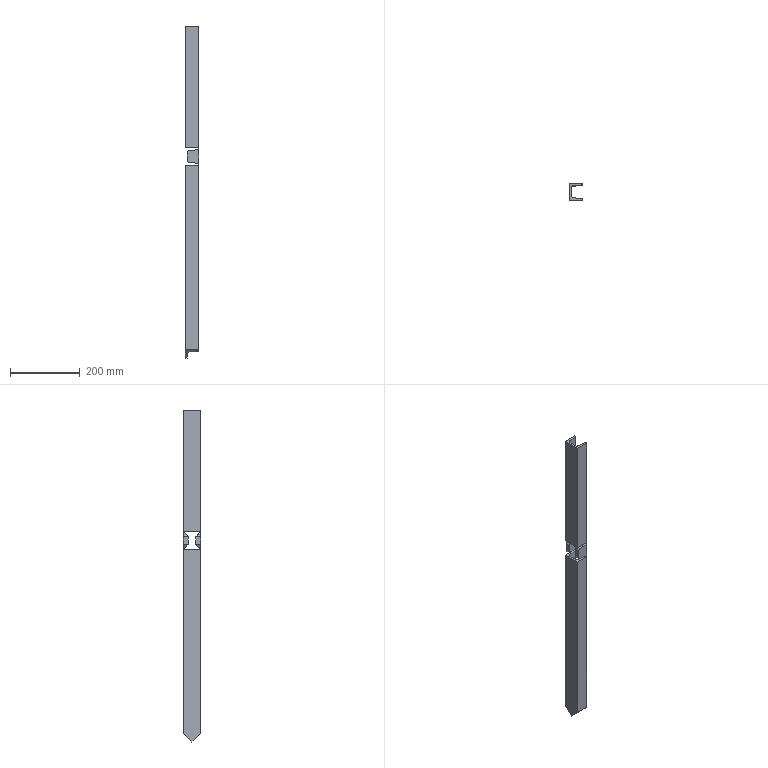Part | STEP file | DIN 1026-1 U 50 1785357074616 | 4 solids | 53 faces | box 38 x 50 x 953.851 mm | volume 646774 mm3 | plane 33 | cylinder 20 | commonest cylinder face diameters 7 x10 14 x10
STEP:
#1=CARTESIAN_POINT('',(38.,25.,556.1));
#2=VERTEX_POINT('',#1);
#3=CARTESIAN_POINT('',(34.779,25.,559.589));
#4=VERTEX_POINT('',#3);
#5=CARTESIAN_POINT('',(34.5,25.,556.1));
#6=DIRECTION('',(0.,-1.,0.));
#7=DIRECTION('',(-0.07975,0.,-0.9968));
#8=AXIS2_PLACEMENT_3D('',#5,#6,#7);
#9=CIRCLE('',#8,3.5);
#10=EDGE_CURVE('',#2,#4,#9,.T.);
#11=ORIENTED_EDGE('',*,*,#10,.F.);
#12=CARTESIAN_POINT('',(38.,22.751,556.1));
#13=VERTEX_POINT('',#12);
#14=CARTESIAN_POINT('',(38.,-253.555,556.1));
#15=DIRECTION('',(0.,1.,0.));
#16=VECTOR('',#15,10.);
#17=LINE('',#14,#16);
#18=EDGE_CURVE('',#13,#2,#17,.T.);
#19=ORIENTED_EDGE('',*,*,#18,.F.);
#20=CARTESIAN_POINT('',(34.779,19.262,559.589));
#21=VERTEX_POINT('',#20);
#22=CARTESIAN_POINT('',(34.5,22.751,556.1));
#23=DIRECTION('',(0.,0.7071,0.7071));
#24=DIRECTION('',(0.,0.7071,-0.7071));
#25=AXIS2_PLACEMENT_3D('',#22,#23,#24);
#26=ELLIPSE('',#25,4.95,3.5);
#27=EDGE_CURVE('',#21,#13,#26,.T.);
#28=ORIENTED_EDGE('',*,*,#27,.F.);
#29=CARTESIAN_POINT('',(34.779,-253.555,559.589));
#30=DIRECTION('',(0.,-1.,0.));
#31=VECTOR('',#30,10.);
#32=LINE('',#29,#31);
#33=EDGE_CURVE('',#4,#21,#32,.T.);
#34=ORIENTED_EDGE('',*,*,#33,.F.);
#35=EDGE_LOOP('',(#11,#19,#28,#34));
#36=FACE_OUTER_BOUND('',#35,.T.);
#37=CARTESIAN_POINT('',(34.5,-253.555,556.1));
#38=DIRECTION('',(0.,1.,0.));
#39=DIRECTION('',(-0.07975,0.,-0.9968));
#40=AXIS2_PLACEMENT_3D('',#37,#38,#39);
#41=CYLINDRICAL_SURFACE('',#40,3.5);
#42=ADVANCED_FACE('',(#36),#41,.F.);
#43=CARTESIAN_POINT('',(11.442,25.,561.456));
#44=VERTEX_POINT('',#43);
#45=CARTESIAN_POINT('',(28.073,25.,560.126));
#46=DIRECTION('',(-0.9968,0.,0.07975));
#47=VECTOR('',#46,10.);
#48=LINE('',#45,#47);
#49=EDGE_CURVE('',#4,#44,#48,.T.);
#50=ORIENTED_EDGE('',*,*,#49,.F.);
#51=ORIENTED_EDGE('',*,*,#33,.T.);
#52=CARTESIAN_POINT('',(11.442,17.395,561.456));
#53=VERTEX_POINT('',#52);
#54=CARTESIAN_POINT('',(34.51,19.241,559.611));
#55=DIRECTION('',(0.9937,0.07949,-0.07949));
#56=VECTOR('',#55,10.);
#57=LINE('',#54,#56);
#58=EDGE_CURVE('',#53,#21,#57,.T.);
#59=ORIENTED_EDGE('',*,*,#58,.F.);
#60=CARTESIAN_POINT('',(11.442,-253.555,561.456));
#61=DIRECTION('',(0.,-1.,0.));
#62=VECTOR('',#61,10.);
#63=LINE('',#60,#62);
#64=EDGE_CURVE('',#44,#53,#63,.T.);
#65=ORIENTED_EDGE('',*,*,#64,.F.);
#66=EDGE_LOOP('',(#50,#51,#59,#65));
#67=FACE_OUTER_BOUND('',#66,.T.);
#68=CARTESIAN_POINT('',(11.442,-253.555,561.456));
#69=DIRECTION('',(0.07975,0.,0.9968));
#70=DIRECTION('',(0.9968,0.,-0.07975));
#71=AXIS2_PLACEMENT_3D('',#68,#69,#70);
#72=PLANE('',#71);
#73=ADVANCED_FACE('',(#67),#72,.F.);
#74=CARTESIAN_POINT('',(5.,25.,568.434));
#75=VERTEX_POINT('',#74);
#76=CARTESIAN_POINT('',(12.,25.,568.434));
#77=DIRECTION('',(0.,1.,0.));
#78=DIRECTION('',(-0.07975,0.,-0.9968));
#79=AXIS2_PLACEMENT_3D('',#76,#77,#78);
#80=CIRCLE('',#79,7.);
#81=EDGE_CURVE('',#44,#75,#80,.T.);
#82=ORIENTED_EDGE('',*,*,#81,.F.);
#83=ORIENTED_EDGE('',*,*,#64,.T.);
#84=CARTESIAN_POINT('',(5.,10.418,568.434));
#85=VERTEX_POINT('',#84);
#86=CARTESIAN_POINT('',(12.,10.418,568.434));
#87=DIRECTION('',(0.,-0.7071,-0.7071));
#88=DIRECTION('',(0.,0.7071,-0.7071));
#89=AXIS2_PLACEMENT_3D('',#86,#87,#88);
#90=ELLIPSE('',#89,9.899,7.);
#91=EDGE_CURVE('',#85,#53,#90,.T.);
#92=ORIENTED_EDGE('',*,*,#91,.F.);
#93=CARTESIAN_POINT('',(5.,-253.555,568.434));
#94=DIRECTION('',(0.,-1.,0.));
#95=VECTOR('',#94,10.);
#96=LINE('',#93,#95);
#97=EDGE_CURVE('',#75,#85,#96,.T.);
#98=ORIENTED_EDGE('',*,*,#97,.F.);
#99=EDGE_LOOP('',(#82,#83,#92,#98));
#100=FACE_OUTER_BOUND('',#99,.T.);
#101=CARTESIAN_POINT('',(12.,-253.555,568.434));
#102=DIRECTION('',(0.,1.,0.));
#103=DIRECTION('',(-0.07975,0.,-0.9968));
#104=AXIS2_PLACEMENT_3D('',#101,#102,#103);
#105=CYLINDRICAL_SURFACE('',#104,7.);
#106=ADVANCED_FACE('',(#100),#105,.T.);
#107=CARTESIAN_POINT('',(5.,25.,589.269));
#108=VERTEX_POINT('',#107);
#109=CARTESIAN_POINT('',(5.,25.,294.634));
#110=DIRECTION('',(0.,0.,1.));
#111=VECTOR('',#110,10.);
#112=LINE('',#109,#111);
#113=EDGE_CURVE('',#75,#108,#112,.T.);
#114=ORIENTED_EDGE('',*,*,#113,.F.);
#115=ORIENTED_EDGE('',*,*,#97,.T.);
#116=CARTESIAN_POINT('',(5.,10.418,589.269));
#117=VERTEX_POINT('',#116);
#118=CARTESIAN_POINT('',(5.,10.418,0.));
#119=DIRECTION('',(0.,0.,1.));
#120=VECTOR('',#119,10.);
#121=LINE('',#118,#120);
#122=EDGE_CURVE('',#85,#117,#121,.T.);
#123=ORIENTED_EDGE('',*,*,#122,.T.);
#124=CARTESIAN_POINT('',(5.,-253.555,589.269));
#125=DIRECTION('',(0.,-1.,0.));
#126=VECTOR('',#125,10.);
#127=LINE('',#124,#126);
#128=EDGE_CURVE('',#108,#117,#127,.T.);
#129=ORIENTED_EDGE('',*,*,#128,.F.);
#130=EDGE_LOOP('',(#114,#115,#123,#129));
#131=FACE_OUTER_BOUND('',#130,.T.);
#132=CARTESIAN_POINT('',(5.,-253.555,589.269));
#133=DIRECTION('',(1.,0.,0.));
#134=DIRECTION('',(0.,0.,-1.));
#135=AXIS2_PLACEMENT_3D('',#132,#133,#134);
#136=PLANE('',#135);
#137=ADVANCED_FACE('',(#131),#136,.F.);
#138=CARTESIAN_POINT('',(11.442,25.,596.247));
#139=VERTEX_POINT('',#138);
#140=CARTESIAN_POINT('',(12.,25.,589.269));
#141=DIRECTION('',(0.,1.,0.));
#142=DIRECTION('',(-1.,0.,0.));
#143=AXIS2_PLACEMENT_3D('',#140,#141,#142);
#144=CIRCLE('',#143,7.);
#145=EDGE_CURVE('',#108,#139,#144,.T.);
#146=ORIENTED_EDGE('',*,*,#145,.F.);
#147=ORIENTED_EDGE('',*,*,#128,.T.);
#148=CARTESIAN_POINT('',(11.442,17.395,596.247));
#149=VERTEX_POINT('',#148);
#150=CARTESIAN_POINT('',(12.,10.418,589.269));
#151=DIRECTION('',(0.,-0.7071,0.7071));
#152=DIRECTION('',(0.,0.7071,0.7071));
#153=AXIS2_PLACEMENT_3D('',#150,#151,#152);
#154=ELLIPSE('',#153,9.899,7.);
#155=EDGE_CURVE('',#149,#117,#154,.T.);
#156=ORIENTED_EDGE('',*,*,#155,.F.);
#157=CARTESIAN_POINT('',(11.442,-253.555,596.247));
#158=DIRECTION('',(0.,-1.,0.));
#159=VECTOR('',#158,10.);
#160=LINE('',#157,#159);
#161=EDGE_CURVE('',#139,#149,#160,.T.);
#162=ORIENTED_EDGE('',*,*,#161,.F.);
#163=EDGE_LOOP('',(#146,#147,#156,#162));
#164=FACE_OUTER_BOUND('',#163,.T.);
#165=CARTESIAN_POINT('',(12.,-253.555,589.269));
#166=DIRECTION('',(0.,1.,0.));
#167=DIRECTION('',(-1.,0.,0.));
#168=AXIS2_PLACEMENT_3D('',#165,#166,#167);
#169=CYLINDRICAL_SURFACE('',#168,7.);
#170=ADVANCED_FACE('',(#164),#169,.T.);
#171=CARTESIAN_POINT('',(34.779,25.,598.114));
#172=VERTEX_POINT('',#171);
#173=CARTESIAN_POINT('',(38.,25.,601.603));
#174=VERTEX_POINT('',#173);
#175=CARTESIAN_POINT('',(34.5,25.,601.603));
#176=DIRECTION('',(0.,-1.,0.));
#177=DIRECTION('',(-1.,0.,0.));
#178=AXIS2_PLACEMENT_3D('',#175,#176,#177);
#179=CIRCLE('',#178,3.5);
#180=EDGE_CURVE('',#172,#174,#179,.T.);
#181=ORIENTED_EDGE('',*,*,#180,.F.);
#182=CARTESIAN_POINT('',(34.779,19.262,598.114));
#183=VERTEX_POINT('',#182);
#184=CARTESIAN_POINT('',(34.779,-253.555,598.114));
#185=DIRECTION('',(0.,-1.,0.));
#186=VECTOR('',#185,10.);
#187=LINE('',#184,#186);
#188=EDGE_CURVE('',#172,#183,#187,.T.);
#189=ORIENTED_EDGE('',*,*,#188,.T.);
#190=CARTESIAN_POINT('',(38.,22.751,601.603));
#191=VERTEX_POINT('',#190);
#192=CARTESIAN_POINT('',(34.5,22.751,601.603));
#193=DIRECTION('',(0.,0.7071,-0.7071));
#194=DIRECTION('',(0.,0.7071,0.7071));
#195=AXIS2_PLACEMENT_3D('',#192,#193,#194);
#196=ELLIPSE('',#195,4.95,3.5);
#197=EDGE_CURVE('',#191,#183,#196,.T.);
#198=ORIENTED_EDGE('',*,*,#197,.F.);
#199=CARTESIAN_POINT('',(38.,-253.555,601.603));
#200=DIRECTION('',(0.,1.,0.));
#201=VECTOR('',#200,10.);
#202=LINE('',#199,#201);
#203=EDGE_CURVE('',#191,#174,#202,.T.);
#204=ORIENTED_EDGE('',*,*,#203,.T.);
#205=EDGE_LOOP('',(#181,#189,#198,#204));
#206=FACE_OUTER_BOUND('',#205,.T.);
#207=CARTESIAN_POINT('',(34.5,-253.555,601.603));
#208=DIRECTION('',(0.,1.,0.));
#209=DIRECTION('',(-1.,0.,0.));
#210=AXIS2_PLACEMENT_3D('',#207,#208,#209);
#211=CYLINDRICAL_SURFACE('',#210,3.5);
#212=ADVANCED_FACE('',(#206),#211,.F.);
#213=CARTESIAN_POINT('',(-6.272,25.,594.83));
#214=DIRECTION('',(0.9968,0.,0.07975));
#215=VECTOR('',#214,10.);
#216=LINE('',#213,#215);
#217=EDGE_CURVE('',#139,#172,#216,.T.);
#218=ORIENTED_EDGE('',*,*,#217,.F.);
#219=ORIENTED_EDGE('',*,*,#161,.T.);
#220=CARTESIAN_POINT('',(0.3821,16.511,595.362));
#221=DIRECTION('',(-0.9937,-0.07949,-0.07949));
#222=VECTOR('',#221,10.);
#223=LINE('',#220,#222);
#224=EDGE_CURVE('',#183,#149,#223,.T.);
#225=ORIENTED_EDGE('',*,*,#224,.F.);
#226=ORIENTED_EDGE('',*,*,#188,.F.);
#227=EDGE_LOOP('',(#218,#219,#225,#226));
#228=FACE_OUTER_BOUND('',#227,.T.);
#229=CARTESIAN_POINT('',(34.779,-253.555,598.114));
#230=DIRECTION('',(0.07975,0.,-0.9968));
#231=DIRECTION('',(-0.9968,0.,-0.07975));
#232=AXIS2_PLACEMENT_3D('',#229,#230,#231);
#233=PLANE('',#232);
#234=ADVANCED_FACE('',(#228),#233,.F.);
#235=ORIENTED_EDGE('',*,*,#10,.T.);
#236=ORIENTED_EDGE('',*,*,#49,.T.);
#237=ORIENTED_EDGE('',*,*,#81,.T.);
#238=ORIENTED_EDGE('',*,*,#113,.T.);
#239=ORIENTED_EDGE('',*,*,#145,.T.);
#240=ORIENTED_EDGE('',*,*,#217,.T.);
#241=ORIENTED_EDGE('',*,*,#180,.T.);
#242=CARTESIAN_POINT('',(38.,25.,0.));
#243=DIRECTION('',(0.,0.,1.));
#244=VECTOR('',#243,10.);
#245=LINE('',#242,#244);
#246=EDGE_CURVE('',#2,#174,#245,.T.);
#247=ORIENTED_EDGE('',*,*,#246,.F.);
#248=EDGE_LOOP('',(#235,#236,#237,#238,#239,#240,#241,#247));
#249=FACE_OUTER_BOUND('',#248,.T.);
#250=CARTESIAN_POINT('',(0.,25.,0.));
#251=DIRECTION('',(0.,1.,0.));
#252=DIRECTION('',(0.,0.,1.));
#253=AXIS2_PLACEMENT_3D('',#250,#251,#252);
#254=PLANE('',#253);
#255=ADVANCED_FACE('',(#249),#254,.T.);
#256=ORIENTED_EDGE('',*,*,#18,.T.);
#257=ORIENTED_EDGE('',*,*,#246,.T.);
#258=ORIENTED_EDGE('',*,*,#203,.F.);
#259=CARTESIAN_POINT('',(38.,22.751,0.));
#260=DIRECTION('',(0.,0.,1.));
#261=VECTOR('',#260,10.);
#262=LINE('',#259,#261);
#263=EDGE_CURVE('',#13,#191,#262,.T.);
#264=ORIENTED_EDGE('',*,*,#263,.F.);
#265=EDGE_LOOP('',(#256,#257,#258,#264));
#266=FACE_OUTER_BOUND('',#265,.T.);
#267=CARTESIAN_POINT('',(38.,25.,0.));
#268=DIRECTION('',(1.,0.,0.));
#269=DIRECTION('',(0.,0.,-1.));
#270=AXIS2_PLACEMENT_3D('',#267,#268,#269);
#271=PLANE('',#270);
#272=ADVANCED_FACE('',(#266),#271,.T.);
#273=ORIENTED_EDGE('',*,*,#91,.T.);
#274=CARTESIAN_POINT('',(11.442,17.395,0.));
#275=DIRECTION('',(0.,0.,1.));
#276=VECTOR('',#275,10.);
#277=LINE('',#274,#276);
#278=EDGE_CURVE('',#53,#149,#277,.T.);
#279=ORIENTED_EDGE('',*,*,#278,.T.);
#280=ORIENTED_EDGE('',*,*,#155,.T.);
#281=ORIENTED_EDGE('',*,*,#122,.F.);
#282=EDGE_LOOP('',(#273,#279,#280,#281));
#283=FACE_OUTER_BOUND('',#282,.T.);
#284=CARTESIAN_POINT('',(12.,10.418,0.));
#285=DIRECTION('',(0.,0.,1.));
#286=DIRECTION('',(-0.07975,0.9968,0.));
#287=AXIS2_PLACEMENT_3D('',#284,#285,#286);
#288=CYLINDRICAL_SURFACE('',#287,7.);
#289=ADVANCED_FACE('',(#283),#288,.F.);
#290=ORIENTED_EDGE('',*,*,#27,.T.);
#291=ORIENTED_EDGE('',*,*,#263,.T.);
#292=ORIENTED_EDGE('',*,*,#197,.T.);
#293=CARTESIAN_POINT('',(34.779,19.262,0.));
#294=DIRECTION('',(0.,0.,1.));
#295=VECTOR('',#294,10.);
#296=LINE('',#293,#295);
#297=EDGE_CURVE('',#21,#183,#296,.T.);
#298=ORIENTED_EDGE('',*,*,#297,.F.);
#299=EDGE_LOOP('',(#290,#291,#292,#298));
#300=FACE_OUTER_BOUND('',#299,.T.);
#301=CARTESIAN_POINT('',(34.5,22.751,0.));
#302=DIRECTION('',(0.,0.,1.));
#303=DIRECTION('',(-0.07975,0.9968,0.));
#304=AXIS2_PLACEMENT_3D('',#301,#302,#303);
#305=CYLINDRICAL_SURFACE('',#304,3.5);
#306=ADVANCED_FACE('',(#300),#305,.T.);
#307=ORIENTED_EDGE('',*,*,#58,.T.);
#308=ORIENTED_EDGE('',*,*,#297,.T.);
#309=ORIENTED_EDGE('',*,*,#224,.T.);
#310=ORIENTED_EDGE('',*,*,#278,.F.);
#311=EDGE_LOOP('',(#307,#308,#309,#310));
#312=FACE_OUTER_BOUND('',#311,.T.);
#313=CARTESIAN_POINT('',(34.779,19.262,0.));
#314=DIRECTION('',(0.07975,-0.9968,0.));
#315=DIRECTION('',(0.,0.,-1.));
#316=AXIS2_PLACEMENT_3D('',#313,#314,#315);
#317=PLANE('',#316);
#318=ADVANCED_FACE('',(#312),#317,.T.);
#319=CLOSED_SHELL('',(#42,#73,#106,#137,#170,#212,#234,#255,#272,#289,#306,#318));
#320=MANIFOLD_SOLID_BREP('',#319);
#321=CARTESIAN_POINT('',(5.,0.,0.));
#322=VERTEX_POINT('',#321);
#323=CARTESIAN_POINT('',(0.,0.,0.));
#324=VERTEX_POINT('',#323);
#325=CARTESIAN_POINT('',(9.5,0.,0.));
#326=DIRECTION('',(-1.,0.,0.));
#327=VECTOR('',#326,10.);
#328=LINE('',#325,#327);
#329=EDGE_CURVE('',#322,#324,#328,.T.);
#330=ORIENTED_EDGE('',*,*,#329,.T.);
#331=CARTESIAN_POINT('',(0.,25.,25.));
#332=VERTEX_POINT('',#331);
#333=CARTESIAN_POINT('',(0.,0.,0.));
#334=DIRECTION('',(0.,-0.7071,-0.7071));
#335=VECTOR('',#334,10.);
#336=LINE('',#333,#335);
#337=EDGE_CURVE('',#332,#324,#336,.T.);
#338=ORIENTED_EDGE('',*,*,#337,.F.);
#339=CARTESIAN_POINT('',(38.,25.,25.));
#340=VERTEX_POINT('',#339);
#341=CARTESIAN_POINT('',(0.,25.,25.));
#342=DIRECTION('',(-1.,0.,0.));
#343=VECTOR('',#342,10.);
#344=LINE('',#341,#343);
#345=EDGE_CURVE('',#340,#332,#344,.T.);
#346=ORIENTED_EDGE('',*,*,#345,.F.);
#347=CARTESIAN_POINT('',(38.,22.751,22.751));
#348=VERTEX_POINT('',#347);
#349=CARTESIAN_POINT('',(38.,6.25,6.25));
#350=DIRECTION('',(0.,0.7071,0.7071));
#351=VECTOR('',#350,10.);
#352=LINE('',#349,#351);
#353=EDGE_CURVE('',#348,#340,#352,.T.);
#354=ORIENTED_EDGE('',*,*,#353,.F.);
#355=CARTESIAN_POINT('',(34.779,19.262,19.262));
#356=VERTEX_POINT('',#355);
#357=CARTESIAN_POINT('',(34.5,22.751,22.751));
#358=DIRECTION('',(0.,-0.7071,0.7071));
#359=DIRECTION('',(0.,0.7071,0.7071));
#360=AXIS2_PLACEMENT_3D('',#357,#358,#359);
#361=ELLIPSE('',#360,4.95,3.5);
#362=EDGE_CURVE('',#356,#348,#361,.T.);
#363=ORIENTED_EDGE('',*,*,#362,.F.);
#364=CARTESIAN_POINT('',(11.442,17.395,17.395));
#365=VERTEX_POINT('',#364);
#366=CARTESIAN_POINT('',(15.327,17.706,17.706));
#367=DIRECTION('',(0.9937,0.07949,0.07949));
#368=VECTOR('',#367,10.);
#369=LINE('',#366,#368);
#370=EDGE_CURVE('',#365,#356,#369,.T.);
#371=ORIENTED_EDGE('',*,*,#370,.F.);
#372=CARTESIAN_POINT('',(5.,10.418,10.418));
#373=VERTEX_POINT('',#372);
#374=CARTESIAN_POINT('',(12.,10.418,10.418));
#375=DIRECTION('',(0.,0.7071,-0.7071));
#376=DIRECTION('',(0.,0.7071,0.7071));
#377=AXIS2_PLACEMENT_3D('',#374,#375,#376);
#378=ELLIPSE('',#377,9.899,7.);
#379=EDGE_CURVE('',#373,#365,#378,.T.);
#380=ORIENTED_EDGE('',*,*,#379,.F.);
#381=CARTESIAN_POINT('',(5.,0.,0.));
#382=DIRECTION('',(0.,0.7071,0.7071));
#383=VECTOR('',#382,10.);
#384=LINE('',#381,#383);
#385=EDGE_CURVE('',#322,#373,#384,.T.);
#386=ORIENTED_EDGE('',*,*,#385,.F.);
#387=EDGE_LOOP('',(#330,#338,#346,#354,#363,#371,#380,#386));
#388=FACE_OUTER_BOUND('',#387,.T.);
#389=CARTESIAN_POINT('',(0.,0.,0.));
#390=DIRECTION('',(0.,-0.7071,0.7071));
#391=DIRECTION('',(1.,0.,0.));
#392=AXIS2_PLACEMENT_3D('',#389,#390,#391);
#393=PLANE('',#392);
#394=ADVANCED_FACE('',(#388),#393,.F.);
#395=ORIENTED_EDGE('',*,*,#353,.T.);
#396=CARTESIAN_POINT('',(38.,25.,553.851));
#397=VERTEX_POINT('',#396);
#398=CARTESIAN_POINT('',(38.,25.,0.));
#399=DIRECTION('',(0.,0.,1.));
#400=VECTOR('',#399,10.);
#401=LINE('',#398,#400);
#402=EDGE_CURVE('',#340,#397,#401,.T.);
#403=ORIENTED_EDGE('',*,*,#402,.T.);
#404=CARTESIAN_POINT('',(38.,22.751,553.851));
#405=VERTEX_POINT('',#404);
#406=CARTESIAN_POINT('',(38.,-114.278,553.851));
#407=DIRECTION('',(0.,-1.,0.));
#408=VECTOR('',#407,10.);
#409=LINE('',#406,#408);
#410=EDGE_CURVE('',#397,#405,#409,.T.);
#411=ORIENTED_EDGE('',*,*,#410,.T.);
#412=CARTESIAN_POINT('',(38.,22.751,0.));
#413=DIRECTION('',(0.,0.,1.));
#414=VECTOR('',#413,10.);
#415=LINE('',#412,#414);
#416=EDGE_CURVE('',#348,#405,#415,.T.);
#417=ORIENTED_EDGE('',*,*,#416,.F.);
#418=EDGE_LOOP('',(#395,#403,#411,#417));
#419=FACE_OUTER_BOUND('',#418,.T.);
#420=CARTESIAN_POINT('',(38.,25.,0.));
#421=DIRECTION('',(1.,0.,0.));
#422=DIRECTION('',(0.,0.,-1.));
#423=AXIS2_PLACEMENT_3D('',#420,#421,#422);
#424=PLANE('',#423);
#425=ADVANCED_FACE('',(#419),#424,.T.);
#426=ORIENTED_EDGE('',*,*,#345,.T.);
#427=CARTESIAN_POINT('',(0.,25.,553.851));
#428=VERTEX_POINT('',#427);
#429=CARTESIAN_POINT('',(0.,25.,0.));
#430=DIRECTION('',(0.,0.,1.));
#431=VECTOR('',#430,10.);
#432=LINE('',#429,#431);
#433=EDGE_CURVE('',#332,#428,#432,.T.);
#434=ORIENTED_EDGE('',*,*,#433,.T.);
#435=CARTESIAN_POINT('',(19.,25.,553.851));
#436=DIRECTION('',(1.,0.,0.));
#437=VECTOR('',#436,10.);
#438=LINE('',#435,#437);
#439=EDGE_CURVE('',#428,#397,#438,.T.);
#440=ORIENTED_EDGE('',*,*,#439,.T.);
#441=ORIENTED_EDGE('',*,*,#402,.F.);
#442=EDGE_LOOP('',(#426,#434,#440,#441));
#443=FACE_OUTER_BOUND('',#442,.T.);
#444=CARTESIAN_POINT('',(0.,25.,0.));
#445=DIRECTION('',(0.,1.,0.));
#446=DIRECTION('',(0.,0.,1.));
#447=AXIS2_PLACEMENT_3D('',#444,#445,#446);
#448=PLANE('',#447);
#449=ADVANCED_FACE('',(#443),#448,.T.);
#450=ORIENTED_EDGE('',*,*,#337,.T.);
#451=CARTESIAN_POINT('',(0.,-25.,25.));
#452=VERTEX_POINT('',#451);
#453=CARTESIAN_POINT('',(0.,0.,0.));
#454=DIRECTION('',(0.,-0.7071,0.7071));
#455=VECTOR('',#454,10.);
#456=LINE('',#453,#455);
#457=EDGE_CURVE('',#324,#452,#456,.T.);
#458=ORIENTED_EDGE('',*,*,#457,.T.);
#459=CARTESIAN_POINT('',(0.,-25.,553.851));
#460=VERTEX_POINT('',#459);
#461=CARTESIAN_POINT('',(0.,-25.,0.));
#462=DIRECTION('',(0.,0.,1.));
#463=VECTOR('',#462,10.);
#464=LINE('',#461,#463);
#465=EDGE_CURVE('',#452,#460,#464,.T.);
#466=ORIENTED_EDGE('',*,*,#465,.T.);
#467=CARTESIAN_POINT('',(0.,-126.778,553.851));
#468=DIRECTION('',(0.,1.,0.));
#469=VECTOR('',#468,10.);
#470=LINE('',#467,#469);
#471=EDGE_CURVE('',#460,#428,#470,.T.);
#472=ORIENTED_EDGE('',*,*,#471,.T.);
#473=ORIENTED_EDGE('',*,*,#433,.F.);
#474=EDGE_LOOP('',(#450,#458,#466,#472,#473));
#475=FACE_OUTER_BOUND('',#474,.T.);
#476=CARTESIAN_POINT('',(0.,0.,0.));
#477=DIRECTION('',(-1.,0.,0.));
#478=DIRECTION('',(0.,0.,1.));
#479=AXIS2_PLACEMENT_3D('',#476,#477,#478);
#480=PLANE('',#479);
#481=ADVANCED_FACE('',(#475),#480,.T.);
#482=ORIENTED_EDGE('',*,*,#385,.T.);
#483=CARTESIAN_POINT('',(5.,10.418,553.851));
#484=VERTEX_POINT('',#483);
#485=CARTESIAN_POINT('',(5.,10.418,0.));
#486=DIRECTION('',(0.,0.,1.));
#487=VECTOR('',#486,10.);
#488=LINE('',#485,#487);
#489=EDGE_CURVE('',#373,#484,#488,.T.);
#490=ORIENTED_EDGE('',*,*,#489,.T.);
#491=CARTESIAN_POINT('',(5.,-10.418,553.851));
#492=VERTEX_POINT('',#491);
#493=CARTESIAN_POINT('',(5.,-126.778,553.851));
#494=DIRECTION('',(0.,-1.,0.));
#495=VECTOR('',#494,10.);
#496=LINE('',#493,#495);
#497=EDGE_CURVE('',#484,#492,#496,.T.);
#498=ORIENTED_EDGE('',*,*,#497,.T.);
#499=CARTESIAN_POINT('',(5.,-10.418,10.418));
#500=VERTEX_POINT('',#499);
#501=CARTESIAN_POINT('',(5.,-10.418,0.));
#502=DIRECTION('',(0.,0.,1.));
#503=VECTOR('',#502,10.);
#504=LINE('',#501,#503);
#505=EDGE_CURVE('',#500,#492,#504,.T.);
#506=ORIENTED_EDGE('',*,*,#505,.F.);
#507=CARTESIAN_POINT('',(5.,0.,0.));
#508=DIRECTION('',(0.,0.7071,-0.7071));
#509=VECTOR('',#508,10.);
#510=LINE('',#507,#509);
#511=EDGE_CURVE('',#500,#322,#510,.T.);
#512=ORIENTED_EDGE('',*,*,#511,.T.);
#513=EDGE_LOOP('',(#482,#490,#498,#506,#512));
#514=FACE_OUTER_BOUND('',#513,.T.);
#515=CARTESIAN_POINT('',(5.,0.,0.));
#516=DIRECTION('',(1.,0.,0.));
#517=DIRECTION('',(0.,0.,-1.));
#518=AXIS2_PLACEMENT_3D('',#515,#516,#517);
#519=PLANE('',#518);
#520=ADVANCED_FACE('',(#514),#519,.T.);
#521=ORIENTED_EDGE('',*,*,#379,.T.);
#522=CARTESIAN_POINT('',(11.442,17.395,553.851));
#523=VERTEX_POINT('',#522);
#524=CARTESIAN_POINT('',(11.442,17.395,0.));
#525=DIRECTION('',(0.,0.,1.));
#526=VECTOR('',#525,10.);
#527=LINE('',#524,#526);
#528=EDGE_CURVE('',#365,#523,#527,.T.);
#529=ORIENTED_EDGE('',*,*,#528,.T.);
#530=CARTESIAN_POINT('',(12.,10.418,553.851));
#531=DIRECTION('',(0.,0.,1.));
#532=DIRECTION('',(-0.07975,0.9968,0.));
#533=AXIS2_PLACEMENT_3D('',#530,#531,#532);
#534=CIRCLE('',#533,7.);
#535=EDGE_CURVE('',#523,#484,#534,.T.);
#536=ORIENTED_EDGE('',*,*,#535,.T.);
#537=ORIENTED_EDGE('',*,*,#489,.F.);
#538=EDGE_LOOP('',(#521,#529,#536,#537));
#539=FACE_OUTER_BOUND('',#538,.T.);
#540=CARTESIAN_POINT('',(12.,10.418,0.));
#541=DIRECTION('',(0.,0.,1.));
#542=DIRECTION('',(-0.07975,0.9968,0.));
#543=AXIS2_PLACEMENT_3D('',#540,#541,#542);
#544=CYLINDRICAL_SURFACE('',#543,7.);
#545=ADVANCED_FACE('',(#539),#544,.F.);
#546=ORIENTED_EDGE('',*,*,#370,.T.);
#547=CARTESIAN_POINT('',(34.779,19.262,553.851));
#548=VERTEX_POINT('',#547);
#549=CARTESIAN_POINT('',(34.779,19.262,0.));
#550=DIRECTION('',(0.,0.,1.));
#551=VECTOR('',#550,10.);
#552=LINE('',#549,#551);
#553=EDGE_CURVE('',#356,#548,#552,.T.);
#554=ORIENTED_EDGE('',*,*,#553,.T.);
#555=CARTESIAN_POINT('',(25.536,18.523,553.851));
#556=DIRECTION('',(-0.9968,-0.07975,0.));
#557=VECTOR('',#556,10.);
#558=LINE('',#555,#557);
#559=EDGE_CURVE('',#548,#523,#558,.T.);
#560=ORIENTED_EDGE('',*,*,#559,.T.);
#561=ORIENTED_EDGE('',*,*,#528,.F.);
#562=EDGE_LOOP('',(#546,#554,#560,#561));
#563=FACE_OUTER_BOUND('',#562,.T.);
#564=CARTESIAN_POINT('',(34.779,19.262,0.));
#565=DIRECTION('',(0.07975,-0.9968,0.));
#566=DIRECTION('',(0.,0.,-1.));
#567=AXIS2_PLACEMENT_3D('',#564,#565,#566);
#568=PLANE('',#567);
#569=ADVANCED_FACE('',(#563),#568,.T.);
#570=ORIENTED_EDGE('',*,*,#362,.T.);
#571=ORIENTED_EDGE('',*,*,#416,.T.);
#572=CARTESIAN_POINT('',(34.5,22.751,553.851));
#573=DIRECTION('',(0.,0.,-1.));
#574=DIRECTION('',(-0.07975,0.9968,0.));
#575=AXIS2_PLACEMENT_3D('',#572,#573,#574);
#576=CIRCLE('',#575,3.5);
#577=EDGE_CURVE('',#405,#548,#576,.T.);
#578=ORIENTED_EDGE('',*,*,#577,.T.);
#579=ORIENTED_EDGE('',*,*,#553,.F.);
#580=EDGE_LOOP('',(#570,#571,#578,#579));
#581=FACE_OUTER_BOUND('',#580,.T.);
#582=CARTESIAN_POINT('',(34.5,22.751,0.));
#583=DIRECTION('',(0.,0.,1.));
#584=DIRECTION('',(-0.07975,0.9968,0.));
#585=AXIS2_PLACEMENT_3D('',#582,#583,#584);
#586=CYLINDRICAL_SURFACE('',#585,3.5);
#587=ADVANCED_FACE('',(#581),#586,.T.);
#588=CARTESIAN_POINT('',(11.442,-17.395,17.395));
#589=VERTEX_POINT('',#588);
#590=CARTESIAN_POINT('',(12.,-10.418,10.418));
#591=DIRECTION('',(0.,-0.7071,-0.7071));
#592=DIRECTION('',(0.,-0.7071,0.7071));
#593=AXIS2_PLACEMENT_3D('',#590,#591,#592);
#594=ELLIPSE('',#593,9.899,7.);
#595=EDGE_CURVE('',#589,#500,#594,.T.);
#596=ORIENTED_EDGE('',*,*,#595,.F.);
#597=CARTESIAN_POINT('',(34.779,-19.262,19.262));
#598=VERTEX_POINT('',#597);
#599=CARTESIAN_POINT('',(3.732,-16.779,16.779));
#600=DIRECTION('',(-0.9937,0.07949,-0.07949));
#601=VECTOR('',#600,10.);
#602=LINE('',#599,#601);
#603=EDGE_CURVE('',#598,#589,#602,.T.);
#604=ORIENTED_EDGE('',*,*,#603,.F.);
#605=CARTESIAN_POINT('',(38.,-22.751,22.751));
#606=VERTEX_POINT('',#605);
#607=CARTESIAN_POINT('',(34.5,-22.751,22.751));
#608=DIRECTION('',(0.,0.7071,0.7071));
#609=DIRECTION('',(0.,-0.7071,0.7071));
#610=AXIS2_PLACEMENT_3D('',#607,#608,#609);
#611=ELLIPSE('',#610,4.95,3.5);
#612=EDGE_CURVE('',#606,#598,#611,.T.);
#613=ORIENTED_EDGE('',*,*,#612,.F.);
#614=CARTESIAN_POINT('',(38.,-25.,25.));
#615=VERTEX_POINT('',#614);
#616=CARTESIAN_POINT('',(38.,-5.688,5.688));
#617=DIRECTION('',(0.,0.7071,-0.7071));
#618=VECTOR('',#617,10.);
#619=LINE('',#616,#618);
#620=EDGE_CURVE('',#615,#606,#619,.T.);
#621=ORIENTED_EDGE('',*,*,#620,.F.);
#622=CARTESIAN_POINT('',(19.,-25.,25.));
#623=DIRECTION('',(1.,0.,0.));
#624=VECTOR('',#623,10.);
#625=LINE('',#622,#624);
#626=EDGE_CURVE('',#452,#615,#625,.T.);
#627=ORIENTED_EDGE('',*,*,#626,.F.);
#628=ORIENTED_EDGE('',*,*,#457,.F.);
#629=ORIENTED_EDGE('',*,*,#329,.F.);
#630=ORIENTED_EDGE('',*,*,#511,.F.);
#631=EDGE_LOOP('',(#596,#604,#613,#621,#627,#628,#629,#630));
#632=FACE_OUTER_BOUND('',#631,.T.);
#633=CARTESIAN_POINT('',(0.,0.,0.));
#634=DIRECTION('',(0.,0.7071,0.7071));
#635=DIRECTION('',(1.,0.,0.));
#636=AXIS2_PLACEMENT_3D('',#633,#634,#635);
#637=PLANE('',#636);
#638=ADVANCED_FACE('',(#632),#637,.F.);
#639=CARTESIAN_POINT('',(11.442,-17.395,553.851));
#640=VERTEX_POINT('',#639);
#641=CARTESIAN_POINT('',(12.,-10.418,553.851));
#642=DIRECTION('',(0.,0.,1.));
#643=DIRECTION('',(-1.,0.,0.));
#644=AXIS2_PLACEMENT_3D('',#641,#642,#643);
#645=CIRCLE('',#644,7.);
#646=EDGE_CURVE('',#492,#640,#645,.T.);
#647=ORIENTED_EDGE('',*,*,#646,.T.);
#648=CARTESIAN_POINT('',(11.442,-17.395,0.));
#649=DIRECTION('',(0.,0.,1.));
#650=VECTOR('',#649,10.);
#651=LINE('',#648,#650);
#652=EDGE_CURVE('',#589,#640,#651,.T.);
#653=ORIENTED_EDGE('',*,*,#652,.F.);
#654=ORIENTED_EDGE('',*,*,#595,.T.);
#655=ORIENTED_EDGE('',*,*,#505,.T.);
#656=EDGE_LOOP('',(#647,#653,#654,#655));
#657=FACE_OUTER_BOUND('',#656,.T.);
#658=CARTESIAN_POINT('',(12.,-10.418,0.));
#659=DIRECTION('',(0.,0.,1.));
#660=DIRECTION('',(-1.,0.,0.));
#661=AXIS2_PLACEMENT_3D('',#658,#659,#660);
#662=CYLINDRICAL_SURFACE('',#661,7.);
#663=ADVANCED_FACE('',(#657),#662,.F.);
#664=CARTESIAN_POINT('',(34.779,-19.262,553.851));
#665=VERTEX_POINT('',#664);
#666=CARTESIAN_POINT('',(34.023,-19.202,553.851));
#667=DIRECTION('',(0.9968,-0.07975,0.));
#668=VECTOR('',#667,10.);
#669=LINE('',#666,#668);
#670=EDGE_CURVE('',#640,#665,#669,.T.);
#671=ORIENTED_EDGE('',*,*,#670,.T.);
#672=CARTESIAN_POINT('',(34.779,-19.262,0.));
#673=DIRECTION('',(0.,0.,1.));
#674=VECTOR('',#673,10.);
#675=LINE('',#672,#674);
#676=EDGE_CURVE('',#598,#665,#675,.T.);
#677=ORIENTED_EDGE('',*,*,#676,.F.);
#678=ORIENTED_EDGE('',*,*,#603,.T.);
#679=ORIENTED_EDGE('',*,*,#652,.T.);
#680=EDGE_LOOP('',(#671,#677,#678,#679));
#681=FACE_OUTER_BOUND('',#680,.T.);
#682=CARTESIAN_POINT('',(11.442,-17.395,0.));
#683=DIRECTION('',(0.07975,0.9968,0.));
#684=DIRECTION('',(0.,0.,1.));
#685=AXIS2_PLACEMENT_3D('',#682,#683,#684);
#686=PLANE('',#685);
#687=ADVANCED_FACE('',(#681),#686,.T.);
#688=CARTESIAN_POINT('',(38.,-22.751,553.851));
#689=VERTEX_POINT('',#688);
#690=CARTESIAN_POINT('',(34.5,-22.751,553.851));
#691=DIRECTION('',(0.,0.,-1.));
#692=DIRECTION('',(-1.,0.,0.));
#693=AXIS2_PLACEMENT_3D('',#690,#691,#692);
#694=CIRCLE('',#693,3.5);
#695=EDGE_CURVE('',#665,#689,#694,.T.);
#696=ORIENTED_EDGE('',*,*,#695,.T.);
#697=CARTESIAN_POINT('',(38.,-22.751,0.));
#698=DIRECTION('',(0.,0.,1.));
#699=VECTOR('',#698,10.);
#700=LINE('',#697,#699);
#701=EDGE_CURVE('',#606,#689,#700,.T.);
#702=ORIENTED_EDGE('',*,*,#701,.F.);
#703=ORIENTED_EDGE('',*,*,#612,.T.);
#704=ORIENTED_EDGE('',*,*,#676,.T.);
#705=EDGE_LOOP('',(#696,#702,#703,#704));
#706=FACE_OUTER_BOUND('',#705,.T.);
#707=CARTESIAN_POINT('',(34.5,-22.751,0.));
#708=DIRECTION('',(0.,0.,1.));
#709=DIRECTION('',(-1.,0.,0.));
#710=AXIS2_PLACEMENT_3D('',#707,#708,#709);
#711=CYLINDRICAL_SURFACE('',#710,3.5);
#712=ADVANCED_FACE('',(#706),#711,.T.);
#713=CARTESIAN_POINT('',(38.,-25.,553.851));
#714=VERTEX_POINT('',#713);
#715=CARTESIAN_POINT('',(38.,-25.,553.851));
#716=DIRECTION('',(-1.,0.,0.));
#717=VECTOR('',#716,10.);
#718=LINE('',#715,#717);
#719=EDGE_CURVE('',#714,#460,#718,.T.);
#720=ORIENTED_EDGE('',*,*,#719,.T.);
#721=ORIENTED_EDGE('',*,*,#465,.F.);
#722=ORIENTED_EDGE('',*,*,#626,.T.);
#723=CARTESIAN_POINT('',(38.,-25.,0.));
#724=DIRECTION('',(0.,0.,1.));
#725=VECTOR('',#724,10.);
#726=LINE('',#723,#725);
#727=EDGE_CURVE('',#615,#714,#726,.T.);
#728=ORIENTED_EDGE('',*,*,#727,.T.);
#729=EDGE_LOOP('',(#720,#721,#722,#728));
#730=FACE_OUTER_BOUND('',#729,.T.);
#731=CARTESIAN_POINT('',(38.,-25.,0.));
#732=DIRECTION('',(0.,-1.,0.));
#733=DIRECTION('',(0.,0.,-1.));
#734=AXIS2_PLACEMENT_3D('',#731,#732,#733);
#735=PLANE('',#734);
#736=ADVANCED_FACE('',(#730),#735,.T.);
#737=CARTESIAN_POINT('',(38.,-138.153,553.851));
#738=DIRECTION('',(0.,-1.,0.));
#739=VECTOR('',#738,10.);
#740=LINE('',#737,#739);
#741=EDGE_CURVE('',#689,#714,#740,.T.);
#742=ORIENTED_EDGE('',*,*,#741,.T.);
#743=ORIENTED_EDGE('',*,*,#727,.F.);
#744=ORIENTED_EDGE('',*,*,#620,.T.);
#745=ORIENTED_EDGE('',*,*,#701,.T.);
#746=EDGE_LOOP('',(#742,#743,#744,#745));
#747=FACE_OUTER_BOUND('',#746,.T.);
#748=CARTESIAN_POINT('',(38.,-22.751,0.));
#749=DIRECTION('',(1.,0.,0.));
#750=DIRECTION('',(0.,0.,-1.));
#751=AXIS2_PLACEMENT_3D('',#748,#749,#750);
#752=PLANE('',#751);
#753=ADVANCED_FACE('',(#747),#752,.T.);
#754=ORIENTED_EDGE('',*,*,#695,.F.);
#755=ORIENTED_EDGE('',*,*,#670,.F.);
#756=ORIENTED_EDGE('',*,*,#646,.F.);
#757=ORIENTED_EDGE('',*,*,#497,.F.);
#758=ORIENTED_EDGE('',*,*,#535,.F.);
#759=ORIENTED_EDGE('',*,*,#559,.F.);
#760=ORIENTED_EDGE('',*,*,#577,.F.);
#761=ORIENTED_EDGE('',*,*,#410,.F.);
#762=ORIENTED_EDGE('',*,*,#439,.F.);
#763=ORIENTED_EDGE('',*,*,#471,.F.);
#764=ORIENTED_EDGE('',*,*,#719,.F.);
#765=ORIENTED_EDGE('',*,*,#741,.F.);
#766=EDGE_LOOP('',(#754,#755,#756,#757,#758,#759,#760,#761,#762,#763,#764,#765));
#767=FACE_OUTER_BOUND('',#766,.T.);
#768=CARTESIAN_POINT('',(38.,-253.555,553.851));
#769=DIRECTION('',(0.,0.,-1.));
#770=DIRECTION('',(-1.,0.,0.));
#771=AXIS2_PLACEMENT_3D('',#768,#769,#770);
#772=PLANE('',#771);
#773=ADVANCED_FACE('',(#767),#772,.F.);
#774=CLOSED_SHELL('',(#394,#425,#449,#481,#520,#545,#569,#587,#638,#663,#687,#712,#736,#753,#773));
#775=MANIFOLD_SOLID_BREP('',#774);
#776=CARTESIAN_POINT('',(34.779,-25.,559.589));
#777=VERTEX_POINT('',#776);
#778=CARTESIAN_POINT('',(38.,-25.,556.1));
#779=VERTEX_POINT('',#778);
#780=CARTESIAN_POINT('',(34.5,-25.,556.1));
#781=DIRECTION('',(0.,1.,0.));
#782=DIRECTION('',(-0.07975,0.,-0.9968));
#783=AXIS2_PLACEMENT_3D('',#780,#781,#782);
#784=CIRCLE('',#783,3.5);
#785=EDGE_CURVE('',#777,#779,#784,.T.);
#786=ORIENTED_EDGE('',*,*,#785,.F.);
#787=CARTESIAN_POINT('',(34.779,-19.262,559.589));
#788=VERTEX_POINT('',#787);
#789=CARTESIAN_POINT('',(34.779,-253.555,559.589));
#790=DIRECTION('',(0.,-1.,0.));
#791=VECTOR('',#790,10.);
#792=LINE('',#789,#791);
#793=EDGE_CURVE('',#788,#777,#792,.T.);
#794=ORIENTED_EDGE('',*,*,#793,.F.);
#795=CARTESIAN_POINT('',(38.,-22.751,556.1));
#796=VERTEX_POINT('',#795);
#797=CARTESIAN_POINT('',(34.5,-22.751,556.1));
#798=DIRECTION('',(0.,-0.7071,0.7071));
#799=DIRECTION('',(0.,-0.7071,-0.7071));
#800=AXIS2_PLACEMENT_3D('',#797,#798,#799);
#801=ELLIPSE('',#800,4.95,3.5);
#802=EDGE_CURVE('',#796,#788,#801,.T.);
#803=ORIENTED_EDGE('',*,*,#802,.F.);
#804=CARTESIAN_POINT('',(38.,-253.555,556.1));
#805=DIRECTION('',(0.,1.,0.));
#806=VECTOR('',#805,10.);
#807=LINE('',#804,#806);
#808=EDGE_CURVE('',#779,#796,#807,.T.);
#809=ORIENTED_EDGE('',*,*,#808,.F.);
#810=EDGE_LOOP('',(#786,#794,#803,#809));
#811=FACE_OUTER_BOUND('',#810,.T.);
#812=CARTESIAN_POINT('',(34.5,-253.555,556.1));
#813=DIRECTION('',(0.,1.,0.));
#814=DIRECTION('',(-0.07975,0.,-0.9968));
#815=AXIS2_PLACEMENT_3D('',#812,#813,#814);
#816=CYLINDRICAL_SURFACE('',#815,3.5);
#817=ADVANCED_FACE('',(#811),#816,.F.);
#818=CARTESIAN_POINT('',(11.442,-25.,561.456));
#819=VERTEX_POINT('',#818);
#820=CARTESIAN_POINT('',(46.952,-25.,558.615));
#821=DIRECTION('',(0.9968,0.,-0.07975));
#822=VECTOR('',#821,10.);
#823=LINE('',#820,#822);
#824=EDGE_CURVE('',#819,#777,#823,.T.);
#825=ORIENTED_EDGE('',*,*,#824,.F.);
#826=CARTESIAN_POINT('',(11.442,-17.395,561.456));
#827=VERTEX_POINT('',#826);
#828=CARTESIAN_POINT('',(11.442,-253.555,561.456));
#829=DIRECTION('',(0.,-1.,0.));
#830=VECTOR('',#829,10.);
#831=LINE('',#828,#830);
#832=EDGE_CURVE('',#827,#819,#831,.T.);
#833=ORIENTED_EDGE('',*,*,#832,.F.);
#834=CARTESIAN_POINT('',(42.943,-19.915,558.936));
#835=DIRECTION('',(-0.9937,0.07949,0.07949));
#836=VECTOR('',#835,10.);
#837=LINE('',#834,#836);
#838=EDGE_CURVE('',#788,#827,#837,.T.);
#839=ORIENTED_EDGE('',*,*,#838,.F.);
#840=ORIENTED_EDGE('',*,*,#793,.T.);
#841=EDGE_LOOP('',(#825,#833,#839,#840));
#842=FACE_OUTER_BOUND('',#841,.T.);
#843=CARTESIAN_POINT('',(11.442,-253.555,561.456));
#844=DIRECTION('',(0.07975,0.,0.9968));
#845=DIRECTION('',(0.9968,0.,-0.07975));
#846=AXIS2_PLACEMENT_3D('',#843,#844,#845);
#847=PLANE('',#846);
#848=ADVANCED_FACE('',(#842),#847,.F.);
#849=CARTESIAN_POINT('',(5.,-25.,568.434));
#850=VERTEX_POINT('',#849);
#851=CARTESIAN_POINT('',(12.,-25.,568.434));
#852=DIRECTION('',(0.,-1.,0.));
#853=DIRECTION('',(-0.07975,0.,-0.9968));
#854=AXIS2_PLACEMENT_3D('',#851,#852,#853);
#855=CIRCLE('',#854,7.);
#856=EDGE_CURVE('',#850,#819,#855,.T.);
#857=ORIENTED_EDGE('',*,*,#856,.F.);
#858=CARTESIAN_POINT('',(5.,-10.418,568.434));
#859=VERTEX_POINT('',#858);
#860=CARTESIAN_POINT('',(5.,-253.555,568.434));
#861=DIRECTION('',(0.,-1.,0.));
#862=VECTOR('',#861,10.);
#863=LINE('',#860,#862);
#864=EDGE_CURVE('',#859,#850,#863,.T.);
#865=ORIENTED_EDGE('',*,*,#864,.F.);
#866=CARTESIAN_POINT('',(12.,-10.418,568.434));
#867=DIRECTION('',(0.,0.7071,-0.7071));
#868=DIRECTION('',(0.,-0.7071,-0.7071));
#869=AXIS2_PLACEMENT_3D('',#866,#867,#868);
#870=ELLIPSE('',#869,9.899,7.);
#871=EDGE_CURVE('',#827,#859,#870,.T.);
#872=ORIENTED_EDGE('',*,*,#871,.F.);
#873=ORIENTED_EDGE('',*,*,#832,.T.);
#874=EDGE_LOOP('',(#857,#865,#872,#873));
#875=FACE_OUTER_BOUND('',#874,.T.);
#876=CARTESIAN_POINT('',(12.,-253.555,568.434));
#877=DIRECTION('',(0.,1.,0.));
#878=DIRECTION('',(-0.07975,0.,-0.9968));
#879=AXIS2_PLACEMENT_3D('',#876,#877,#878);
#880=CYLINDRICAL_SURFACE('',#879,7.);
#881=ADVANCED_FACE('',(#875),#880,.T.);
#882=CARTESIAN_POINT('',(34.779,-25.,598.114));
#883=VERTEX_POINT('',#882);
#884=CARTESIAN_POINT('',(11.442,-25.,596.247));
#885=VERTEX_POINT('',#884);
#886=CARTESIAN_POINT('',(12.607,-25.,596.34));
#887=DIRECTION('',(-0.9968,0.,-0.07975));
#888=VECTOR('',#887,10.);
#889=LINE('',#886,#888);
#890=EDGE_CURVE('',#883,#885,#889,.T.);
#891=ORIENTED_EDGE('',*,*,#890,.F.);
#892=CARTESIAN_POINT('',(34.779,-19.262,598.114));
#893=VERTEX_POINT('',#892);
#894=CARTESIAN_POINT('',(34.779,-253.555,598.114));
#895=DIRECTION('',(0.,-1.,0.));
#896=VECTOR('',#895,10.);
#897=LINE('',#894,#896);
#898=EDGE_CURVE('',#893,#883,#897,.T.);
#899=ORIENTED_EDGE('',*,*,#898,.F.);
#900=CARTESIAN_POINT('',(11.442,-17.395,596.247));
#901=VERTEX_POINT('',#900);
#902=CARTESIAN_POINT('',(8.815,-17.185,596.037));
#903=DIRECTION('',(0.9937,-0.07949,0.07949));
#904=VECTOR('',#903,10.);
#905=LINE('',#902,#904);
#906=EDGE_CURVE('',#901,#893,#905,.T.);
#907=ORIENTED_EDGE('',*,*,#906,.F.);
#908=CARTESIAN_POINT('',(11.442,-253.555,596.247));
#909=DIRECTION('',(0.,-1.,0.));
#910=VECTOR('',#909,10.);
#911=LINE('',#908,#910);
#912=EDGE_CURVE('',#901,#885,#911,.T.);
#913=ORIENTED_EDGE('',*,*,#912,.T.);
#914=EDGE_LOOP('',(#891,#899,#907,#913));
#915=FACE_OUTER_BOUND('',#914,.T.);
#916=CARTESIAN_POINT('',(34.779,-253.555,598.114));
#917=DIRECTION('',(0.07975,0.,-0.9968));
#918=DIRECTION('',(-0.9968,0.,-0.07975));
#919=AXIS2_PLACEMENT_3D('',#916,#917,#918);
#920=PLANE('',#919);
#921=ADVANCED_FACE('',(#915),#920,.F.);
#922=CARTESIAN_POINT('',(38.,-25.,601.603));
#923=VERTEX_POINT('',#922);
#924=CARTESIAN_POINT('',(34.5,-25.,601.603));
#925=DIRECTION('',(0.,1.,0.));
#926=DIRECTION('',(-1.,0.,0.));
#927=AXIS2_PLACEMENT_3D('',#924,#925,#926);
#928=CIRCLE('',#927,3.5);
#929=EDGE_CURVE('',#923,#883,#928,.T.);
#930=ORIENTED_EDGE('',*,*,#929,.F.);
#931=CARTESIAN_POINT('',(38.,-22.751,601.603));
#932=VERTEX_POINT('',#931);
#933=CARTESIAN_POINT('',(38.,-253.555,601.603));
#934=DIRECTION('',(0.,1.,0.));
#935=VECTOR('',#934,10.);
#936=LINE('',#933,#935);
#937=EDGE_CURVE('',#923,#932,#936,.T.);
#938=ORIENTED_EDGE('',*,*,#937,.T.);
#939=CARTESIAN_POINT('',(34.5,-22.751,601.603));
#940=DIRECTION('',(0.,-0.7071,-0.7071));
#941=DIRECTION('',(0.,-0.7071,0.7071));
#942=AXIS2_PLACEMENT_3D('',#939,#940,#941);
#943=ELLIPSE('',#942,4.95,3.5);
#944=EDGE_CURVE('',#893,#932,#943,.T.);
#945=ORIENTED_EDGE('',*,*,#944,.F.);
#946=ORIENTED_EDGE('',*,*,#898,.T.);
#947=EDGE_LOOP('',(#930,#938,#945,#946));
#948=FACE_OUTER_BOUND('',#947,.T.);
#949=CARTESIAN_POINT('',(34.5,-253.555,601.603));
#950=DIRECTION('',(0.,1.,0.));
#951=DIRECTION('',(-1.,0.,0.));
#952=AXIS2_PLACEMENT_3D('',#949,#950,#951);
#953=CYLINDRICAL_SURFACE('',#952,3.5);
#954=ADVANCED_FACE('',(#948),#953,.F.);
#955=CARTESIAN_POINT('',(5.,-25.,589.269));
#956=VERTEX_POINT('',#955);
#957=CARTESIAN_POINT('',(5.,-25.,294.634));
#958=DIRECTION('',(0.,0.,-1.));
#959=VECTOR('',#958,10.);
#960=LINE('',#957,#959);
#961=EDGE_CURVE('',#956,#850,#960,.T.);
#962=ORIENTED_EDGE('',*,*,#961,.F.);
#963=CARTESIAN_POINT('',(5.,-10.418,589.269));
#964=VERTEX_POINT('',#963);
#965=CARTESIAN_POINT('',(5.,-253.555,589.269));
#966=DIRECTION('',(0.,-1.,0.));
#967=VECTOR('',#966,10.);
#968=LINE('',#965,#967);
#969=EDGE_CURVE('',#964,#956,#968,.T.);
#970=ORIENTED_EDGE('',*,*,#969,.F.);
#971=CARTESIAN_POINT('',(5.,-10.418,0.));
#972=DIRECTION('',(0.,0.,1.));
#973=VECTOR('',#972,10.);
#974=LINE('',#971,#973);
#975=EDGE_CURVE('',#859,#964,#974,.T.);
#976=ORIENTED_EDGE('',*,*,#975,.F.);
#977=ORIENTED_EDGE('',*,*,#864,.T.);
#978=EDGE_LOOP('',(#962,#970,#976,#977));
#979=FACE_OUTER_BOUND('',#978,.T.);
#980=CARTESIAN_POINT('',(5.,-253.555,589.269));
#981=DIRECTION('',(1.,0.,0.));
#982=DIRECTION('',(0.,0.,-1.));
#983=AXIS2_PLACEMENT_3D('',#980,#981,#982);
#984=PLANE('',#983);
#985=ADVANCED_FACE('',(#979),#984,.F.);
#986=CARTESIAN_POINT('',(12.,-25.,589.269));
#987=DIRECTION('',(0.,-1.,0.));
#988=DIRECTION('',(-1.,0.,0.));
#989=AXIS2_PLACEMENT_3D('',#986,#987,#988);
#990=CIRCLE('',#989,7.);
#991=EDGE_CURVE('',#885,#956,#990,.T.);
#992=ORIENTED_EDGE('',*,*,#991,.F.);
#993=ORIENTED_EDGE('',*,*,#912,.F.);
#994=CARTESIAN_POINT('',(12.,-10.418,589.269));
#995=DIRECTION('',(0.,0.7071,0.7071));
#996=DIRECTION('',(0.,-0.7071,0.7071));
#997=AXIS2_PLACEMENT_3D('',#994,#995,#996);
#998=ELLIPSE('',#997,9.899,7.);
#999=EDGE_CURVE('',#964,#901,#998,.T.);
#1000=ORIENTED_EDGE('',*,*,#999,.F.);
#1001=ORIENTED_EDGE('',*,*,#969,.T.);
#1002=EDGE_LOOP('',(#992,#993,#1000,#1001));
#1003=FACE_OUTER_BOUND('',#1002,.T.);
#1004=CARTESIAN_POINT('',(12.,-253.555,589.269));
#1005=DIRECTION('',(0.,1.,0.));
#1006=DIRECTION('',(-1.,0.,0.));
#1007=AXIS2_PLACEMENT_3D('',#1004,#1005,#1006);
#1008=CYLINDRICAL_SURFACE('',#1007,7.);
#1009=ADVANCED_FACE('',(#1003),#1008,.T.);
#1010=ORIENTED_EDGE('',*,*,#808,.T.);
#1011=CARTESIAN_POINT('',(38.,-22.751,0.));
#1012=DIRECTION('',(0.,0.,1.));
#1013=VECTOR('',#1012,10.);
#1014=LINE('',#1011,#1013);
#1015=EDGE_CURVE('',#796,#932,#1014,.T.);
#1016=ORIENTED_EDGE('',*,*,#1015,.T.);
#1017=ORIENTED_EDGE('',*,*,#937,.F.);
#1018=CARTESIAN_POINT('',(38.,-25.,0.));
#1019=DIRECTION('',(0.,0.,1.));
#1020=VECTOR('',#1019,10.);
#1021=LINE('',#1018,#1020);
#1022=EDGE_CURVE('',#779,#923,#1021,.T.);
#1023=ORIENTED_EDGE('',*,*,#1022,.F.);
#1024=EDGE_LOOP('',(#1010,#1016,#1017,#1023));
#1025=FACE_OUTER_BOUND('',#1024,.T.);
#1026=CARTESIAN_POINT('',(38.,-22.751,0.));
#1027=DIRECTION('',(1.,0.,0.));
#1028=DIRECTION('',(0.,0.,-1.));
#1029=AXIS2_PLACEMENT_3D('',#1026,#1027,#1028);
#1030=PLANE('',#1029);
#1031=ADVANCED_FACE('',(#1025),#1030,.T.);
#1032=ORIENTED_EDGE('',*,*,#802,.T.);
#1033=CARTESIAN_POINT('',(34.779,-19.262,0.));
#1034=DIRECTION('',(0.,0.,1.));
#1035=VECTOR('',#1034,10.);
#1036=LINE('',#1033,#1035);
#1037=EDGE_CURVE('',#788,#893,#1036,.T.);
#1038=ORIENTED_EDGE('',*,*,#1037,.T.);
#1039=ORIENTED_EDGE('',*,*,#944,.T.);
#1040=ORIENTED_EDGE('',*,*,#1015,.F.);
#1041=EDGE_LOOP('',(#1032,#1038,#1039,#1040));
#1042=FACE_OUTER_BOUND('',#1041,.T.);
#1043=CARTESIAN_POINT('',(34.5,-22.751,0.));
#1044=DIRECTION('',(0.,0.,1.));
#1045=DIRECTION('',(-1.,0.,0.));
#1046=AXIS2_PLACEMENT_3D('',#1043,#1044,#1045);
#1047=CYLINDRICAL_SURFACE('',#1046,3.5);
#1048=ADVANCED_FACE('',(#1042),#1047,.T.);
#1049=ORIENTED_EDGE('',*,*,#838,.T.);
#1050=CARTESIAN_POINT('',(11.442,-17.395,0.));
#1051=DIRECTION('',(0.,0.,1.));
#1052=VECTOR('',#1051,10.);
#1053=LINE('',#1050,#1052);
#1054=EDGE_CURVE('',#827,#901,#1053,.T.);
#1055=ORIENTED_EDGE('',*,*,#1054,.T.);
#1056=ORIENTED_EDGE('',*,*,#906,.T.);
#1057=ORIENTED_EDGE('',*,*,#1037,.F.);
#1058=EDGE_LOOP('',(#1049,#1055,#1056,#1057));
#1059=FACE_OUTER_BOUND('',#1058,.T.);
#1060=CARTESIAN_POINT('',(11.442,-17.395,0.));
#1061=DIRECTION('',(0.07975,0.9968,0.));
#1062=DIRECTION('',(0.,0.,1.));
#1063=AXIS2_PLACEMENT_3D('',#1060,#1061,#1062);
#1064=PLANE('',#1063);
#1065=ADVANCED_FACE('',(#1059),#1064,.T.);
#1066=ORIENTED_EDGE('',*,*,#871,.T.);
#1067=ORIENTED_EDGE('',*,*,#975,.T.);
#1068=ORIENTED_EDGE('',*,*,#999,.T.);
#1069=ORIENTED_EDGE('',*,*,#1054,.F.);
#1070=EDGE_LOOP('',(#1066,#1067,#1068,#1069));
#1071=FACE_OUTER_BOUND('',#1070,.T.);
#1072=CARTESIAN_POINT('',(12.,-10.418,0.));
#1073=DIRECTION('',(0.,0.,1.));
#1074=DIRECTION('',(-1.,0.,0.));
#1075=AXIS2_PLACEMENT_3D('',#1072,#1073,#1074);
#1076=CYLINDRICAL_SURFACE('',#1075,7.);
#1077=ADVANCED_FACE('',(#1071),#1076,.F.);
#1078=ORIENTED_EDGE('',*,*,#785,.T.);
#1079=ORIENTED_EDGE('',*,*,#1022,.T.);
#1080=ORIENTED_EDGE('',*,*,#929,.T.);
#1081=ORIENTED_EDGE('',*,*,#890,.T.);
#1082=ORIENTED_EDGE('',*,*,#991,.T.);
#1083=ORIENTED_EDGE('',*,*,#961,.T.);
#1084=ORIENTED_EDGE('',*,*,#856,.T.);
#1085=ORIENTED_EDGE('',*,*,#824,.T.);
#1086=EDGE_LOOP('',(#1078,#1079,#1080,#1081,#1082,#1083,#1084,#1085));
#1087=FACE_OUTER_BOUND('',#1086,.T.);
#1088=CARTESIAN_POINT('',(38.,-25.,0.));
#1089=DIRECTION('',(0.,-1.,0.));
#1090=DIRECTION('',(0.,0.,-1.));
#1091=AXIS2_PLACEMENT_3D('',#1088,#1089,#1090);
#1092=PLANE('',#1091);
#1093=ADVANCED_FACE('',(#1087),#1092,.T.);
#1094=CLOSED_SHELL('',(#817,#848,#881,#921,#954,#985,#1009,#1031,#1048,#1065,#1077,#1093));
#1095=MANIFOLD_SOLID_BREP('',#1094);
#1096=CARTESIAN_POINT('',(0.,25.,953.851));
#1097=VERTEX_POINT('',#1096);
#1098=CARTESIAN_POINT('',(38.,25.,953.851));
#1099=VERTEX_POINT('',#1098);
#1100=CARTESIAN_POINT('',(9.5,25.,953.851));
#1101=DIRECTION('',(1.,0.,0.));
#1102=VECTOR('',#1101,10.);
#1103=LINE('',#1100,#1102);
#1104=EDGE_CURVE('',#1097,#1099,#1103,.T.);
#1105=ORIENTED_EDGE('',*,*,#1104,.F.);
#1106=CARTESIAN_POINT('',(0.,-25.,953.851));
#1107=VERTEX_POINT('',#1106);
#1108=CARTESIAN_POINT('',(0.,0.,953.851));
#1109=DIRECTION('',(0.,1.,0.));
#1110=VECTOR('',#1109,10.);
#1111=LINE('',#1108,#1110);
#1112=EDGE_CURVE('',#1107,#1097,#1111,.T.);
#1113=ORIENTED_EDGE('',*,*,#1112,.F.);
#1114=CARTESIAN_POINT('',(38.,-25.,953.851));
#1115=VERTEX_POINT('',#1114);
#1116=CARTESIAN_POINT('',(28.5,-25.,953.851));
#1117=DIRECTION('',(-1.,0.,0.));
#1118=VECTOR('',#1117,10.);
#1119=LINE('',#1116,#1118);
#1120=EDGE_CURVE('',#1115,#1107,#1119,.T.);
#1121=ORIENTED_EDGE('',*,*,#1120,.F.);
#1122=CARTESIAN_POINT('',(38.,-22.751,953.851));
#1123=VERTEX_POINT('',#1122);
#1124=CARTESIAN_POINT('',(38.,-11.376,953.851));
#1125=DIRECTION('',(0.,-1.,0.));
#1126=VECTOR('',#1125,10.);
#1127=LINE('',#1124,#1126);
#1128=EDGE_CURVE('',#1123,#1115,#1127,.T.);
#1129=ORIENTED_EDGE('',*,*,#1128,.F.);
#1130=CARTESIAN_POINT('',(34.779,-19.262,953.851));
#1131=VERTEX_POINT('',#1130);
#1132=CARTESIAN_POINT('',(34.5,-22.751,953.851));
#1133=DIRECTION('',(0.,0.,-1.));
#1134=DIRECTION('',(-1.,0.,0.));
#1135=AXIS2_PLACEMENT_3D('',#1132,#1133,#1134);
#1136=CIRCLE('',#1135,3.5);
#1137=EDGE_CURVE('',#1131,#1123,#1136,.T.);
#1138=ORIENTED_EDGE('',*,*,#1137,.F.);
#1139=CARTESIAN_POINT('',(11.442,-17.395,953.851));
#1140=VERTEX_POINT('',#1139);
#1141=CARTESIAN_POINT('',(14.505,-17.64,953.851));
#1142=DIRECTION('',(0.9968,-0.07975,0.));
#1143=VECTOR('',#1142,10.);
#1144=LINE('',#1141,#1143);
#1145=EDGE_CURVE('',#1140,#1131,#1144,.T.);
#1146=ORIENTED_EDGE('',*,*,#1145,.F.);
#1147=CARTESIAN_POINT('',(5.,-10.418,953.851));
#1148=VERTEX_POINT('',#1147);
#1149=CARTESIAN_POINT('',(12.,-10.418,953.851));
#1150=DIRECTION('',(0.,0.,1.));
#1151=DIRECTION('',(-1.,0.,0.));
#1152=AXIS2_PLACEMENT_3D('',#1149,#1150,#1151);
#1153=CIRCLE('',#1152,7.);
#1154=EDGE_CURVE('',#1148,#1140,#1153,.T.);
#1155=ORIENTED_EDGE('',*,*,#1154,.F.);
#1156=CARTESIAN_POINT('',(5.,10.418,953.851));
#1157=VERTEX_POINT('',#1156);
#1158=CARTESIAN_POINT('',(5.,0.,953.851));
#1159=DIRECTION('',(0.,-1.,0.));
#1160=VECTOR('',#1159,10.);
#1161=LINE('',#1158,#1160);
#1162=EDGE_CURVE('',#1157,#1148,#1161,.T.);
#1163=ORIENTED_EDGE('',*,*,#1162,.F.);
#1164=CARTESIAN_POINT('',(11.442,17.395,953.851));
#1165=VERTEX_POINT('',#1164);
#1166=CARTESIAN_POINT('',(12.,10.418,953.851));
#1167=DIRECTION('',(0.,0.,1.));
#1168=DIRECTION('',(-0.07975,0.9968,0.));
#1169=AXIS2_PLACEMENT_3D('',#1166,#1167,#1168);
#1170=CIRCLE('',#1169,7.);
#1171=EDGE_CURVE('',#1165,#1157,#1170,.T.);
#1172=ORIENTED_EDGE('',*,*,#1171,.F.);
#1173=CARTESIAN_POINT('',(34.779,19.262,953.851));
#1174=VERTEX_POINT('',#1173);
#1175=CARTESIAN_POINT('',(26.174,18.574,953.851));
#1176=DIRECTION('',(-0.9968,-0.07975,0.));
#1177=VECTOR('',#1176,10.);
#1178=LINE('',#1175,#1177);
#1179=EDGE_CURVE('',#1174,#1165,#1178,.T.);
#1180=ORIENTED_EDGE('',*,*,#1179,.F.);
#1181=CARTESIAN_POINT('',(38.,22.751,953.851));
#1182=VERTEX_POINT('',#1181);
#1183=CARTESIAN_POINT('',(34.5,22.751,953.851));
#1184=DIRECTION('',(0.,0.,-1.));
#1185=DIRECTION('',(-0.07975,0.9968,0.));
#1186=AXIS2_PLACEMENT_3D('',#1183,#1184,#1185);
#1187=CIRCLE('',#1186,3.5);
#1188=EDGE_CURVE('',#1182,#1174,#1187,.T.);
#1189=ORIENTED_EDGE('',*,*,#1188,.F.);
#1190=CARTESIAN_POINT('',(38.,12.5,953.851));
#1191=DIRECTION('',(0.,-1.,0.));
#1192=VECTOR('',#1191,10.);
#1193=LINE('',#1190,#1192);
#1194=EDGE_CURVE('',#1099,#1182,#1193,.T.);
#1195=ORIENTED_EDGE('',*,*,#1194,.F.);
#1196=EDGE_LOOP('',(#1105,#1113,#1121,#1129,#1138,#1146,#1155,#1163,#1172,#1180,#1189,#1195));
#1197=FACE_OUTER_BOUND('',#1196,.T.);
#1198=CARTESIAN_POINT('',(19.,0.,953.851));
#1199=DIRECTION('',(0.,0.,1.));
#1200=DIRECTION('',(1.,0.,0.));
#1201=AXIS2_PLACEMENT_3D('',#1198,#1199,#1200);
#1202=PLANE('',#1201);
#1203=ADVANCED_FACE('',(#1197),#1202,.T.);
#1204=CARTESIAN_POINT('',(11.442,17.395,603.851));
#1205=VERTEX_POINT('',#1204);
#1206=CARTESIAN_POINT('',(34.779,19.262,603.851));
#1207=VERTEX_POINT('',#1206);
#1208=CARTESIAN_POINT('',(6.657,17.013,603.851));
#1209=DIRECTION('',(0.9968,0.07975,0.));
#1210=VECTOR('',#1209,10.);
#1211=LINE('',#1208,#1210);
#1212=EDGE_CURVE('',#1205,#1207,#1211,.T.);
#1213=ORIENTED_EDGE('',*,*,#1212,.T.);
#1214=CARTESIAN_POINT('',(34.779,19.262,0.));
#1215=DIRECTION('',(0.,0.,1.));
#1216=VECTOR('',#1215,10.);
#1217=LINE('',#1214,#1216);
#1218=EDGE_CURVE('',#1207,#1174,#1217,.T.);
#1219=ORIENTED_EDGE('',*,*,#1218,.T.);
#1220=ORIENTED_EDGE('',*,*,#1179,.T.);
#1221=CARTESIAN_POINT('',(11.442,17.395,0.));
#1222=DIRECTION('',(0.,0.,1.));
#1223=VECTOR('',#1222,10.);
#1224=LINE('',#1221,#1223);
#1225=EDGE_CURVE('',#1205,#1165,#1224,.T.);
#1226=ORIENTED_EDGE('',*,*,#1225,.F.);
#1227=EDGE_LOOP('',(#1213,#1219,#1220,#1226));
#1228=FACE_OUTER_BOUND('',#1227,.T.);
#1229=CARTESIAN_POINT('',(34.779,19.262,0.));
#1230=DIRECTION('',(0.07975,-0.9968,0.));
#1231=DIRECTION('',(0.,0.,-1.));
#1232=AXIS2_PLACEMENT_3D('',#1229,#1230,#1231);
#1233=PLANE('',#1232);
#1234=ADVANCED_FACE('',(#1228),#1233,.T.);
#1235=CARTESIAN_POINT('',(38.,22.751,603.851));
#1236=VERTEX_POINT('',#1235);
#1237=CARTESIAN_POINT('',(34.5,22.751,603.851));
#1238=DIRECTION('',(0.,0.,1.));
#1239=DIRECTION('',(-0.07975,0.9968,0.));
#1240=AXIS2_PLACEMENT_3D('',#1237,#1238,#1239);
#1241=CIRCLE('',#1240,3.5);
#1242=EDGE_CURVE('',#1207,#1236,#1241,.T.);
#1243=ORIENTED_EDGE('',*,*,#1242,.T.);
#1244=CARTESIAN_POINT('',(38.,22.751,0.));
#1245=DIRECTION('',(0.,0.,1.));
#1246=VECTOR('',#1245,10.);
#1247=LINE('',#1244,#1246);
#1248=EDGE_CURVE('',#1236,#1182,#1247,.T.);
#1249=ORIENTED_EDGE('',*,*,#1248,.T.);
#1250=ORIENTED_EDGE('',*,*,#1188,.T.);
#1251=ORIENTED_EDGE('',*,*,#1218,.F.);
#1252=EDGE_LOOP('',(#1243,#1249,#1250,#1251));
#1253=FACE_OUTER_BOUND('',#1252,.T.);
#1254=CARTESIAN_POINT('',(34.5,22.751,0.));
#1255=DIRECTION('',(0.,0.,1.));
#1256=DIRECTION('',(-0.07975,0.9968,0.));
#1257=AXIS2_PLACEMENT_3D('',#1254,#1255,#1256);
#1258=CYLINDRICAL_SURFACE('',#1257,3.5);
#1259=ADVANCED_FACE('',(#1253),#1258,.T.);
#1260=CARTESIAN_POINT('',(5.,10.418,603.851));
#1261=VERTEX_POINT('',#1260);
#1262=CARTESIAN_POINT('',(12.,10.418,603.851));
#1263=DIRECTION('',(0.,0.,-1.));
#1264=DIRECTION('',(-0.07975,0.9968,0.));
#1265=AXIS2_PLACEMENT_3D('',#1262,#1263,#1264);
#1266=CIRCLE('',#1265,7.);
#1267=EDGE_CURVE('',#1261,#1205,#1266,.T.);
#1268=ORIENTED_EDGE('',*,*,#1267,.T.);
#1269=ORIENTED_EDGE('',*,*,#1225,.T.);
#1270=ORIENTED_EDGE('',*,*,#1171,.T.);
#1271=CARTESIAN_POINT('',(5.,10.418,0.));
#1272=DIRECTION('',(0.,0.,1.));
#1273=VECTOR('',#1272,10.);
#1274=LINE('',#1271,#1273);
#1275=EDGE_CURVE('',#1261,#1157,#1274,.T.);
#1276=ORIENTED_EDGE('',*,*,#1275,.F.);
#1277=EDGE_LOOP('',(#1268,#1269,#1270,#1276));
#1278=FACE_OUTER_BOUND('',#1277,.T.);
#1279=CARTESIAN_POINT('',(12.,10.418,0.));
#1280=DIRECTION('',(0.,0.,1.));
#1281=DIRECTION('',(-0.07975,0.9968,0.));
#1282=AXIS2_PLACEMENT_3D('',#1279,#1280,#1281);
#1283=CYLINDRICAL_SURFACE('',#1282,7.);
#1284=ADVANCED_FACE('',(#1278),#1283,.F.);
#1285=CARTESIAN_POINT('',(38.,25.,603.851));
#1286=VERTEX_POINT('',#1285);
#1287=CARTESIAN_POINT('',(38.,-114.278,603.851));
#1288=DIRECTION('',(0.,1.,0.));
#1289=VECTOR('',#1288,10.);
#1290=LINE('',#1287,#1289);
#1291=EDGE_CURVE('',#1236,#1286,#1290,.T.);
#1292=ORIENTED_EDGE('',*,*,#1291,.T.);
#1293=CARTESIAN_POINT('',(38.,25.,0.));
#1294=DIRECTION('',(0.,0.,1.));
#1295=VECTOR('',#1294,10.);
#1296=LINE('',#1293,#1295);
#1297=EDGE_CURVE('',#1286,#1099,#1296,.T.);
#1298=ORIENTED_EDGE('',*,*,#1297,.T.);
#1299=ORIENTED_EDGE('',*,*,#1194,.T.);
#1300=ORIENTED_EDGE('',*,*,#1248,.F.);
#1301=EDGE_LOOP('',(#1292,#1298,#1299,#1300));
#1302=FACE_OUTER_BOUND('',#1301,.T.);
#1303=CARTESIAN_POINT('',(38.,25.,0.));
#1304=DIRECTION('',(1.,0.,0.));
#1305=DIRECTION('',(0.,0.,-1.));
#1306=AXIS2_PLACEMENT_3D('',#1303,#1304,#1305);
#1307=PLANE('',#1306);
#1308=ADVANCED_FACE('',(#1302),#1307,.T.);
#1309=CARTESIAN_POINT('',(5.,-10.418,603.851));
#1310=VERTEX_POINT('',#1309);
#1311=CARTESIAN_POINT('',(5.,-126.778,603.851));
#1312=DIRECTION('',(0.,1.,0.));
#1313=VECTOR('',#1312,10.);
#1314=LINE('',#1311,#1313);
#1315=EDGE_CURVE('',#1310,#1261,#1314,.T.);
#1316=ORIENTED_EDGE('',*,*,#1315,.T.);
#1317=ORIENTED_EDGE('',*,*,#1275,.T.);
#1318=ORIENTED_EDGE('',*,*,#1162,.T.);
#1319=CARTESIAN_POINT('',(5.,-10.418,0.));
#1320=DIRECTION('',(0.,0.,1.));
#1321=VECTOR('',#1320,10.);
#1322=LINE('',#1319,#1321);
#1323=EDGE_CURVE('',#1310,#1148,#1322,.T.);
#1324=ORIENTED_EDGE('',*,*,#1323,.F.);
#1325=EDGE_LOOP('',(#1316,#1317,#1318,#1324));
#1326=FACE_OUTER_BOUND('',#1325,.T.);
#1327=CARTESIAN_POINT('',(5.,0.,0.));
#1328=DIRECTION('',(1.,0.,0.));
#1329=DIRECTION('',(0.,0.,-1.));
#1330=AXIS2_PLACEMENT_3D('',#1327,#1328,#1329);
#1331=PLANE('',#1330);
#1332=ADVANCED_FACE('',(#1326),#1331,.T.);
#1333=CARTESIAN_POINT('',(11.442,-17.395,603.851));
#1334=VERTEX_POINT('',#1333);
#1335=CARTESIAN_POINT('',(12.,-10.418,603.851));
#1336=DIRECTION('',(0.,0.,-1.));
#1337=DIRECTION('',(-1.,0.,0.));
#1338=AXIS2_PLACEMENT_3D('',#1335,#1336,#1337);
#1339=CIRCLE('',#1338,7.);
#1340=EDGE_CURVE('',#1334,#1310,#1339,.T.);
#1341=ORIENTED_EDGE('',*,*,#1340,.T.);
#1342=ORIENTED_EDGE('',*,*,#1323,.T.);
#1343=ORIENTED_EDGE('',*,*,#1154,.T.);
#1344=CARTESIAN_POINT('',(11.442,-17.395,0.));
#1345=DIRECTION('',(0.,0.,1.));
#1346=VECTOR('',#1345,10.);
#1347=LINE('',#1344,#1346);
#1348=EDGE_CURVE('',#1334,#1140,#1347,.T.);
#1349=ORIENTED_EDGE('',*,*,#1348,.F.);
#1350=EDGE_LOOP('',(#1341,#1342,#1343,#1349));
#1351=FACE_OUTER_BOUND('',#1350,.T.);
#1352=CARTESIAN_POINT('',(12.,-10.418,0.));
#1353=DIRECTION('',(0.,0.,1.));
#1354=DIRECTION('',(-1.,0.,0.));
#1355=AXIS2_PLACEMENT_3D('',#1352,#1353,#1354);
#1356=CYLINDRICAL_SURFACE('',#1355,7.);
#1357=ADVANCED_FACE('',(#1351),#1356,.F.);
#1358=CARTESIAN_POINT('',(0.,25.,603.851));
#1359=VERTEX_POINT('',#1358);
#1360=CARTESIAN_POINT('',(0.,25.,603.851));
#1361=DIRECTION('',(-1.,0.,0.));
#1362=VECTOR('',#1361,10.);
#1363=LINE('',#1360,#1362);
#1364=EDGE_CURVE('',#1286,#1359,#1363,.T.);
#1365=ORIENTED_EDGE('',*,*,#1364,.T.);
#1366=CARTESIAN_POINT('',(0.,25.,0.));
#1367=DIRECTION('',(0.,0.,1.));
#1368=VECTOR('',#1367,10.);
#1369=LINE('',#1366,#1368);
#1370=EDGE_CURVE('',#1359,#1097,#1369,.T.);
#1371=ORIENTED_EDGE('',*,*,#1370,.T.);
#1372=ORIENTED_EDGE('',*,*,#1104,.T.);
#1373=ORIENTED_EDGE('',*,*,#1297,.F.);
#1374=EDGE_LOOP('',(#1365,#1371,#1372,#1373));
#1375=FACE_OUTER_BOUND('',#1374,.T.);
#1376=CARTESIAN_POINT('',(0.,25.,0.));
#1377=DIRECTION('',(0.,1.,0.));
#1378=DIRECTION('',(0.,0.,1.));
#1379=AXIS2_PLACEMENT_3D('',#1376,#1377,#1378);
#1380=PLANE('',#1379);
#1381=ADVANCED_FACE('',(#1375),#1380,.T.);
#1382=CARTESIAN_POINT('',(34.779,-19.262,603.851));
#1383=VERTEX_POINT('',#1382);
#1384=CARTESIAN_POINT('',(15.144,-17.691,603.851));
#1385=DIRECTION('',(-0.9968,0.07975,0.));
#1386=VECTOR('',#1385,10.);
#1387=LINE('',#1384,#1386);
#1388=EDGE_CURVE('',#1383,#1334,#1387,.T.);
#1389=ORIENTED_EDGE('',*,*,#1388,.T.);
#1390=ORIENTED_EDGE('',*,*,#1348,.T.);
#1391=ORIENTED_EDGE('',*,*,#1145,.T.);
#1392=CARTESIAN_POINT('',(34.779,-19.262,0.));
#1393=DIRECTION('',(0.,0.,1.));
#1394=VECTOR('',#1393,10.);
#1395=LINE('',#1392,#1394);
#1396=EDGE_CURVE('',#1383,#1131,#1395,.T.);
#1397=ORIENTED_EDGE('',*,*,#1396,.F.);
#1398=EDGE_LOOP('',(#1389,#1390,#1391,#1397));
#1399=FACE_OUTER_BOUND('',#1398,.T.);
#1400=CARTESIAN_POINT('',(11.442,-17.395,0.));
#1401=DIRECTION('',(0.07975,0.9968,0.));
#1402=DIRECTION('',(0.,0.,1.));
#1403=AXIS2_PLACEMENT_3D('',#1400,#1401,#1402);
#1404=PLANE('',#1403);
#1405=ADVANCED_FACE('',(#1399),#1404,.T.);
#1406=CARTESIAN_POINT('',(0.,-25.,603.851));
#1407=VERTEX_POINT('',#1406);
#1408=CARTESIAN_POINT('',(0.,-126.778,603.851));
#1409=DIRECTION('',(0.,-1.,0.));
#1410=VECTOR('',#1409,10.);
#1411=LINE('',#1408,#1410);
#1412=EDGE_CURVE('',#1359,#1407,#1411,.T.);
#1413=ORIENTED_EDGE('',*,*,#1412,.T.);
#1414=CARTESIAN_POINT('',(0.,-25.,0.));
#1415=DIRECTION('',(0.,0.,1.));
#1416=VECTOR('',#1415,10.);
#1417=LINE('',#1414,#1416);
#1418=EDGE_CURVE('',#1407,#1107,#1417,.T.);
#1419=ORIENTED_EDGE('',*,*,#1418,.T.);
#1420=ORIENTED_EDGE('',*,*,#1112,.T.);
#1421=ORIENTED_EDGE('',*,*,#1370,.F.);
#1422=EDGE_LOOP('',(#1413,#1419,#1420,#1421));
#1423=FACE_OUTER_BOUND('',#1422,.T.);
#1424=CARTESIAN_POINT('',(0.,0.,0.));
#1425=DIRECTION('',(-1.,0.,0.));
#1426=DIRECTION('',(0.,0.,1.));
#1427=AXIS2_PLACEMENT_3D('',#1424,#1425,#1426);
#1428=PLANE('',#1427);
#1429=ADVANCED_FACE('',(#1423),#1428,.T.);
#1430=CARTESIAN_POINT('',(38.,-22.751,603.851));
#1431=VERTEX_POINT('',#1430);
#1432=CARTESIAN_POINT('',(34.5,-22.751,603.851));
#1433=DIRECTION('',(0.,0.,1.));
#1434=DIRECTION('',(-1.,0.,0.));
#1435=AXIS2_PLACEMENT_3D('',#1432,#1433,#1434);
#1436=CIRCLE('',#1435,3.5);
#1437=EDGE_CURVE('',#1431,#1383,#1436,.T.);
#1438=ORIENTED_EDGE('',*,*,#1437,.T.);
#1439=ORIENTED_EDGE('',*,*,#1396,.T.);
#1440=ORIENTED_EDGE('',*,*,#1137,.T.);
#1441=CARTESIAN_POINT('',(38.,-22.751,0.));
#1442=DIRECTION('',(0.,0.,1.));
#1443=VECTOR('',#1442,10.);
#1444=LINE('',#1441,#1443);
#1445=EDGE_CURVE('',#1431,#1123,#1444,.T.);
#1446=ORIENTED_EDGE('',*,*,#1445,.F.);
#1447=EDGE_LOOP('',(#1438,#1439,#1440,#1446));
#1448=FACE_OUTER_BOUND('',#1447,.T.);
#1449=CARTESIAN_POINT('',(34.5,-22.751,0.));
#1450=DIRECTION('',(0.,0.,1.));
#1451=DIRECTION('',(-1.,0.,0.));
#1452=AXIS2_PLACEMENT_3D('',#1449,#1450,#1451);
#1453=CYLINDRICAL_SURFACE('',#1452,3.5);
#1454=ADVANCED_FACE('',(#1448),#1453,.T.);
#1455=CARTESIAN_POINT('',(38.,-25.,603.851));
#1456=VERTEX_POINT('',#1455);
#1457=CARTESIAN_POINT('',(19.,-25.,603.851));
#1458=DIRECTION('',(1.,0.,0.));
#1459=VECTOR('',#1458,10.);
#1460=LINE('',#1457,#1459);
#1461=EDGE_CURVE('',#1407,#1456,#1460,.T.);
#1462=ORIENTED_EDGE('',*,*,#1461,.T.);
#1463=CARTESIAN_POINT('',(38.,-25.,0.));
#1464=DIRECTION('',(0.,0.,1.));
#1465=VECTOR('',#1464,10.);
#1466=LINE('',#1463,#1465);
#1467=EDGE_CURVE('',#1456,#1115,#1466,.T.);
#1468=ORIENTED_EDGE('',*,*,#1467,.T.);
#1469=ORIENTED_EDGE('',*,*,#1120,.T.);
#1470=ORIENTED_EDGE('',*,*,#1418,.F.);
#1471=EDGE_LOOP('',(#1462,#1468,#1469,#1470));
#1472=FACE_OUTER_BOUND('',#1471,.T.);
#1473=CARTESIAN_POINT('',(38.,-25.,0.));
#1474=DIRECTION('',(0.,-1.,0.));
#1475=DIRECTION('',(0.,0.,-1.));
#1476=AXIS2_PLACEMENT_3D('',#1473,#1474,#1475);
#1477=PLANE('',#1476);
#1478=ADVANCED_FACE('',(#1472),#1477,.T.);
#1479=CARTESIAN_POINT('',(38.,-138.153,603.851));
#1480=DIRECTION('',(0.,1.,0.));
#1481=VECTOR('',#1480,10.);
#1482=LINE('',#1479,#1481);
#1483=EDGE_CURVE('',#1456,#1431,#1482,.T.);
#1484=ORIENTED_EDGE('',*,*,#1483,.T.);
#1485=ORIENTED_EDGE('',*,*,#1445,.T.);
#1486=ORIENTED_EDGE('',*,*,#1128,.T.);
#1487=ORIENTED_EDGE('',*,*,#1467,.F.);
#1488=EDGE_LOOP('',(#1484,#1485,#1486,#1487));
#1489=FACE_OUTER_BOUND('',#1488,.T.);
#1490=CARTESIAN_POINT('',(38.,-22.751,0.));
#1491=DIRECTION('',(1.,0.,0.));
#1492=DIRECTION('',(0.,0.,-1.));
#1493=AXIS2_PLACEMENT_3D('',#1490,#1491,#1492);
#1494=PLANE('',#1493);
#1495=ADVANCED_FACE('',(#1489),#1494,.T.);
#1496=ORIENTED_EDGE('',*,*,#1437,.F.);
#1497=ORIENTED_EDGE('',*,*,#1483,.F.);
#1498=ORIENTED_EDGE('',*,*,#1461,.F.);
#1499=ORIENTED_EDGE('',*,*,#1412,.F.);
#1500=ORIENTED_EDGE('',*,*,#1364,.F.);
#1501=ORIENTED_EDGE('',*,*,#1291,.F.);
#1502=ORIENTED_EDGE('',*,*,#1242,.F.);
#1503=ORIENTED_EDGE('',*,*,#1212,.F.);
#1504=ORIENTED_EDGE('',*,*,#1267,.F.);
#1505=ORIENTED_EDGE('',*,*,#1315,.F.);
#1506=ORIENTED_EDGE('',*,*,#1340,.F.);
#1507=ORIENTED_EDGE('',*,*,#1388,.F.);
#1508=EDGE_LOOP('',(#1496,#1497,#1498,#1499,#1500,#1501,#1502,#1503,#1504,#1505,#1506,#1507));
#1509=FACE_OUTER_BOUND('',#1508,.T.);
#1510=CARTESIAN_POINT('',(0.,-253.555,603.851));
#1511=DIRECTION('',(0.,0.,1.));
#1512=DIRECTION('',(1.,0.,0.));
#1513=AXIS2_PLACEMENT_3D('',#1510,#1511,#1512);
#1514=PLANE('',#1513);
#1515=ADVANCED_FACE('',(#1509),#1514,.F.);
#1516=CLOSED_SHELL('',(#1203,#1234,#1259,#1284,#1308,#1332,#1357,#1381,#1405,#1429,#1454,#1478,#1495,#1515));
#1517=MANIFOLD_SOLID_BREP('',#1516);
#1518=(LENGTH_UNIT()NAMED_UNIT(*)SI_UNIT(.MILLI.,.METRE.));
#1519=UNCERTAINTY_MEASURE_WITH_UNIT(LENGTH_MEASURE(0.01),#1518,'','');
#1520=(NAMED_UNIT(*)PLANE_ANGLE_UNIT()SI_UNIT($,.RADIAN.));
#1521=(NAMED_UNIT(*)SI_UNIT($,.STERADIAN.)SOLID_ANGLE_UNIT());
#1522=(GEOMETRIC_REPRESENTATION_CONTEXT(3)GLOBAL_UNCERTAINTY_ASSIGNED_CONTEXT((#1519))GLOBAL_UNIT_ASSIGNED_CONTEXT((#1518,#1520,#1521))REPRESENTATION_CONTEXT('',''));
#1523=ADVANCED_BREP_SHAPE_REPRESENTATION('',(#320,#775,#1095,#1517),#1522);